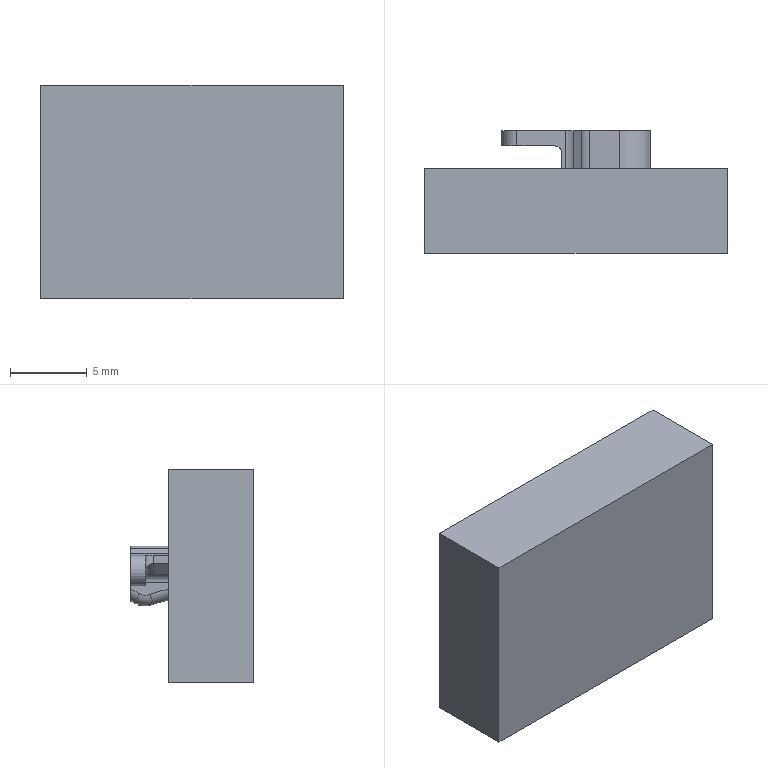NC program | NX | posted with a generic post | part box 19.7 x 8 x 13.91 mm
Lines 6971 to 7835 of 12778:
(ZLEVEL_PROFILE_COPY_1 , TOOL : D2)
N13910 T02 M6
N13912 G54
N13914 G17 G0 G90 X1.619 Y-2.755 B0. C0. S6500 M3
N13916 G43 Z30. H2
N13918 Z-0.04
N13920 G94 G1 X1.446 Y-2.455 F1000.
N13922 G3 X1.273 Y-2.355 R0.2
N13924 G1 X0.696 F1200.
N13926 X0.202 Y-2.652
N13928 G3 X0.105 Y-2.826 R0.2
N13930 G1 X0.111 Y-3.151
N13932 G0 X1.619 Y-2.755 Z-0.08
N13934 G1 X1.446 Y-2.455 F1000.
N13936 G3 X1.273 Y-2.355 R0.2
N13938 G1 X0.696 F1200.
N13940 X0.202 Y-2.652
N13942 G3 X0.105 Y-2.826 R0.2
N13944 G1 X0.111 Y-3.151
N13946 G0 X1.619 Y-2.755 Z-0.12
N13948 G1 X1.446 Y-2.455 F1000.
N13950 G3 X1.273 Y-2.355 R0.2
N13952 G1 X0.696 F1200.
N13954 X0.202 Y-2.652
N13956 G3 X0.105 Y-2.826 R0.2
N13958 G1 X0.111 Y-3.151
N13960 G0 X1.619 Y-2.755 Z-0.16
N13962 G1 X1.446 Y-2.455 F1000.
N13964 G3 X1.273 Y-2.355 R0.2
N13966 G1 X0.696 F1200.
N13968 X0.202 Y-2.652
N13970 G3 X0.105 Y-2.826 R0.2
N13972 G1 X0.111 Y-3.151
N13974 G0 X1.619 Y-2.755 Z-0.2
N13976 G1 X1.446 Y-2.455 F1000.
N13978 G3 X1.273 Y-2.355 R0.2
N13980 G1 X0.696 F1200.
N13982 X0.202 Y-2.652
N13984 G3 X0.105 Y-2.826 R0.2
N13986 G1 X0.111 Y-3.151
N13988 G0 X1.619 Y-2.755 Z-0.24
N13990 G1 X1.446 Y-2.455 F1000.
N13992 G3 X1.273 Y-2.355 R0.2
N13994 G1 X0.696 F1200.
N13996 X0.202 Y-2.652
N13998 G3 X0.105 Y-2.826 R0.2
N14000 G1 X0.111 Y-3.151
N14002 G0 X1.619 Y-2.755 Z-0.28
N14004 G1 X1.446 Y-2.455 F1000.
N14006 G3 X1.273 Y-2.355 R0.2
N14008 G1 X0.696 F1200.
N14010 X0.202 Y-2.652
N14012 G3 X0.105 Y-2.826 R0.2
N14014 G1 X0.111 Y-3.151
N14016 G0 X1.619 Y-2.755 Z-0.32
N14018 G1 X1.446 Y-2.455 F1000.
N14020 G3 X1.273 Y-2.355 R0.2
N14022 G1 X0.696 F1200.
N14024 X0.202 Y-2.652
N14026 G3 X0.105 Y-2.826 R0.2
N14028 G1 X0.111 Y-3.151
N14030 G0 X1.619 Y-2.755 Z-0.36
N14032 G1 X1.446 Y-2.455 F1000.
N14034 G3 X1.273 Y-2.355 R0.2
N14036 G1 X0.696 F1200.
N14038 X0.202 Y-2.652
N14040 G3 X0.105 Y-2.826 R0.2
N14042 G1 X0.111 Y-3.151
N14044 G0 X1.619 Y-2.755 Z-0.4
N14046 G1 X1.446 Y-2.455 F1000.
N14048 G3 X1.273 Y-2.355 R0.2
N14050 G1 X0.696 F1200.
N14052 X0.202 Y-2.652
N14054 G3 X0.105 Y-2.826 R0.2
N14056 G1 X0.111 Y-3.151
N14058 G0 X1.619 Y-2.755 Z-0.44
N14060 G1 X1.446 Y-2.455 F1000.
N14062 G3 X1.273 Y-2.355 R0.2
N14064 G1 X0.696 F1200.
N14066 X0.202 Y-2.652
N14068 G3 X0.105 Y-2.826 R0.2
N14070 G1 X0.111 Y-3.151
N14072 G0 X1.619 Y-2.755 Z-0.48
N14074 G1 X1.446 Y-2.455 F1000.
N14076 G3 X1.273 Y-2.355 R0.2
N14078 G1 X0.696 F1200.
N14080 X0.202 Y-2.652
N14082 G3 X0.105 Y-2.826 R0.2
N14084 G1 X0.111 Y-3.151
N14086 G0 X1.619 Y-2.755 Z-0.52
N14088 G1 X1.446 Y-2.455 F1000.
N14090 G3 X1.273 Y-2.355 R0.2
N14092 G1 X0.696 F1200.
N14094 X0.202 Y-2.652
N14096 G3 X0.105 Y-2.826 R0.2
N14098 G1 X0.111 Y-3.151
N14100 G0 X1.619 Y-2.755 Z-0.56
N14102 G1 X1.446 Y-2.455 F1000.
N14104 G3 X1.273 Y-2.355 R0.2
N14106 G1 X0.696 F1200.
N14108 X0.202 Y-2.652
N14110 G3 X0.105 Y-2.826 R0.2
N14112 G1 X0.111 Y-3.151
N14114 G0 X1.619 Y-2.755 Z-0.6
N14116 G1 X1.446 Y-2.455 F1000.
N14118 G3 X1.273 Y-2.355 R0.2
N14120 G1 X0.696 F1200.
N14122 X0.202 Y-2.652
N14124 G3 X0.105 Y-2.826 R0.2
N14126 G1 X0.111 Y-3.151
N14128 G0 X1.619 Y-2.755 Z-0.64
N14130 G1 X1.446 Y-2.455 F1000.
N14132 G3 X1.273 Y-2.355 R0.2
N14134 G1 X0.696 F1200.
N14136 X0.202 Y-2.652
N14138 G3 X0.105 Y-2.826 R0.2
N14140 G1 X0.111 Y-3.151
N14142 G0 X1.619 Y-2.755 Z-0.68
N14144 G1 X1.446 Y-2.455 F1000.
N14146 G3 X1.273 Y-2.355 R0.2
N14148 G1 X0.696 F1200.
N14150 X0.202 Y-2.652
N14152 G3 X0.105 Y-2.826 R0.2
N14154 G1 X0.111 Y-3.151
N14156 G0 X1.619 Y-2.755 Z-0.72
N14158 G1 X1.446 Y-2.455 F1000.
N14160 G3 X1.273 Y-2.355 R0.2
N14162 G1 X0.696 F1200.
N14164 X0.202 Y-2.652
N14166 G3 X0.105 Y-2.826 R0.2
N14168 G1 X0.111 Y-3.151
N14170 G0 X1.619 Y-2.755 Z-0.76
N14172 G1 X1.446 Y-2.455 F1000.
N14174 G3 X1.273 Y-2.355 R0.2
N14176 G1 X0.696 F1200.
N14178 X0.202 Y-2.652
N14180 G3 X0.105 Y-2.826 R0.2
N14182 G1 X0.111 Y-3.151
N14184 G0 X1.619 Y-2.755 Z-0.8
N14186 G1 X1.446 Y-2.455 F1000.
N14188 G3 X1.273 Y-2.355 R0.2
N14190 G1 X0.696 F1200.
N14192 X0.202 Y-2.652
N14194 G3 X0.105 Y-2.826 R0.2
N14196 G1 X0.111 Y-3.151
N14198 G0 X1.619 Y-2.755 Z-0.84
N14200 G1 X1.446 Y-2.455 F1000.
N14202 G3 X1.273 Y-2.355 R0.2
N14204 G1 X0.696 F1200.
N14206 X0.202 Y-2.652
N14208 G3 X0.105 Y-2.826 R0.2
N14210 G1 X0.111 Y-3.151
N14212 G0 X1.619 Y-2.755 Z-0.88
N14214 G1 X1.446 Y-2.455 F1000.
N14216 G3 X1.273 Y-2.355 R0.2
N14218 G1 X0.696 F1200.
N14220 X0.202 Y-2.652
N14222 G3 X0.105 Y-2.826 R0.2
N14224 G1 X0.111 Y-3.151
N14226 G0 X1.619 Y-2.755 Z-0.92
N14228 G1 X1.446 Y-2.455 F1000.
N14230 G3 X1.273 Y-2.355 R0.2
N14232 G1 X0.696 F1200.
N14234 X0.202 Y-2.652
N14236 G3 X0.105 Y-2.826 R0.2
N14238 G1 X0.111 Y-3.151
N14240 G0 X1.619 Y-2.755 Z-0.96
N14242 G1 X1.446 Y-2.455 F1000.
N14244 G3 X1.273 Y-2.355 R0.2
N14246 G1 X0.696 F1200.
N14248 X0.202 Y-2.652
N14250 G3 X0.105 Y-2.826 R0.2
N14252 G1 X0.111 Y-3.151
N14254 G0 X1.619 Y-2.755 Z-1.
N14256 G1 X1.446 Y-2.455 F1000.
N14258 G3 X1.273 Y-2.355 R0.2
N14260 G1 X0.696 F1200.
N14262 X0.202 Y-2.652
N14264 G3 X0.105 Y-2.826 R0.2
N14266 G1 X0.111 Y-3.151
N14268 G0 X1.619 Y-2.755 Z-1.04
N14270 G1 X1.446 Y-2.455 F1000.
N14272 G3 X1.273 Y-2.355 R0.2
N14274 G1 X0.696 F1200.
N14276 X0.202 Y-2.652
N14278 G3 X0.105 Y-2.826 R0.2
N14280 G1 X0.111 Y-3.151
N14282 G0 X1.619 Y-2.755 Z-1.08
N14284 G1 X1.446 Y-2.455 F1000.
N14286 G3 X1.273 Y-2.355 R0.2
N14288 G1 X0.696 F1200.
N14290 X0.202 Y-2.652
N14292 G3 X0.105 Y-2.826 R0.2
N14294 G1 X0.111 Y-3.151
N14296 G0 X1.619 Y-2.755 Z-1.12
N14298 G1 X1.446 Y-2.455 F1000.
N14300 G3 X1.273 Y-2.355 R0.2
N14302 G1 X0.696 F1200.
N14304 X0.202 Y-2.652
N14306 G3 X0.105 Y-2.826 R0.2
N14308 G1 X0.111 Y-3.151
N14310 G0 X1.619 Y-2.755 Z-1.16
N14312 G1 X1.446 Y-2.455 F1000.
N14314 G3 X1.273 Y-2.355 R0.2
N14316 G1 X0.696 F1200.
N14318 X0.202 Y-2.652
N14320 G3 X0.105 Y-2.826 R0.2
N14322 G1 X0.111 Y-3.151
N14324 G0 X1.619 Y-2.755 Z-1.2
N14326 G1 X1.446 Y-2.455 F1000.
N14328 G3 X1.273 Y-2.355 R0.2
N14330 G1 X0.696 F1200.
N14332 X0.202 Y-2.652
N14334 G3 X0.105 Y-2.826 R0.2
N14336 G1 X0.111 Y-3.151
N14338 G0 X1.619 Y-2.755 Z-1.24
N14340 G1 X1.446 Y-2.455 F1000.
N14342 G3 X1.273 Y-2.355 R0.2
N14344 G1 X0.696 F1200.
N14346 X0.202 Y-2.652
N14348 G3 X0.105 Y-2.826 R0.2
N14350 G1 X0.111 Y-3.151
N14352 G0 X1.619 Y-2.755 Z-1.28
N14354 G1 X1.446 Y-2.455 F1000.
N14356 G3 X1.273 Y-2.355 R0.2
N14358 G1 X0.696 F1200.
N14360 X0.202 Y-2.652
N14362 G3 X0.105 Y-2.826 R0.2
N14364 G1 X0.111 Y-3.151
N14366 G0 X1.619 Y-2.755 Z-1.32
N14368 G1 X1.446 Y-2.455 F1000.
N14370 G3 X1.273 Y-2.355 R0.2
N14372 G1 X0.696 F1200.
N14374 X0.202 Y-2.652
N14376 G3 X0.105 Y-2.826 R0.2
N14378 G1 X0.111 Y-3.151
N14380 G0 X1.619 Y-2.755 Z-1.36
N14382 G1 X1.446 Y-2.455 F1000.
N14384 G3 X1.273 Y-2.355 R0.2
N14386 G1 X0.696 F1200.
N14388 X0.202 Y-2.652
N14390 G3 X0.105 Y-2.826 R0.2
N14392 G1 X0.111 Y-3.151
N14394 G0 X1.619 Y-2.755 Z-1.4
N14396 G1 X1.446 Y-2.455 F1000.
N14398 G3 X1.273 Y-2.355 R0.2
N14400 G1 X0.696 F1200.
N14402 X0.202 Y-2.652
N14404 G3 X0.105 Y-2.826 R0.2
N14406 G1 X0.111 Y-3.151
N14408 G0 X1.619 Y-2.755 Z-1.44
N14410 G1 X1.446 Y-2.455 F1000.
N14412 G3 X1.273 Y-2.355 R0.2
N14414 G1 X0.696 F1200.
N14416 X0.202 Y-2.652
N14418 G3 X0.105 Y-2.826 R0.2
N14420 G1 X0.111 Y-3.151
N14422 G0 X1.619 Y-2.755 Z-1.48
N14424 G1 X1.446 Y-2.455 F1000.
N14426 G3 X1.273 Y-2.355 R0.2
N14428 G1 X0.696 F1200.
N14430 X0.202 Y-2.652
N14432 G3 X0.105 Y-2.826 R0.2
N14434 G1 X0.111 Y-3.151
N14436 G0 X1.619 Y-2.755 Z-1.52
N14438 G1 X1.446 Y-2.455 F1000.
N14440 G3 X1.273 Y-2.355 R0.2
N14442 G1 X0.696 F1200.
N14444 X0.202 Y-2.652
N14446 G3 X0.105 Y-2.826 R0.2
N14448 G1 X0.111 Y-3.151
N14450 G0 X1.619 Y-2.755 Z-1.56
N14452 G1 X1.446 Y-2.455 F1000.
N14454 G3 X1.273 Y-2.355 R0.2
N14456 G1 X0.696 F1200.
N14458 X0.202 Y-2.652
N14460 G3 X0.105 Y-2.826 R0.2
N14462 G1 X0.111 Y-3.151
N14464 G0 X1.619 Y-2.755 Z-1.6
N14466 G1 X1.446 Y-2.455 F1000.
N14468 G3 X1.273 Y-2.355 R0.2
N14470 G1 X0.696 F1200.
N14472 X0.202 Y-2.652
N14474 G3 X0.105 Y-2.826 R0.2
N14476 G1 X0.111 Y-3.151
N14478 G0 X1.619 Y-2.755 Z-1.64
N14480 G1 X1.446 Y-2.455 F1000.
N14482 G3 X1.273 Y-2.355 R0.2
N14484 G1 X0.696 F1200.
N14486 X0.202 Y-2.652
N14488 G3 X0.105 Y-2.826 R0.2
N14490 G1 X0.111 Y-3.151
N14492 G0 X1.619 Y-2.755 Z-1.68
N14494 G1 X1.446 Y-2.455 F1000.
N14496 G3 X1.273 Y-2.355 R0.2
N14498 G1 X0.696 F1200.
N14500 X0.202 Y-2.652
N14502 G3 X0.105 Y-2.826 R0.2
N14504 G1 X0.111 Y-3.151
N14506 G0 X1.619 Y-2.755 Z-1.72
N14508 G1 X1.446 Y-2.455 F1000.
N14510 G3 X1.273 Y-2.355 R0.2
N14512 G1 X0.696 F1200.
N14514 X0.202 Y-2.652
N14516 G3 X0.105 Y-2.826 R0.2
N14518 G1 X0.111 Y-3.151
N14520 G0 X1.619 Y-2.755 Z-1.76
N14522 G1 X1.446 Y-2.455 F1000.
N14524 G3 X1.273 Y-2.355 R0.2
N14526 G1 X0.696 F1200.
N14528 X0.202 Y-2.652
N14530 G3 X0.105 Y-2.826 R0.2
N14532 G1 X0.111 Y-3.151
N14534 G0 X1.619 Y-2.755 Z-1.8
N14536 G1 X1.446 Y-2.455 F1000.
N14538 G3 X1.273 Y-2.355 R0.2
N14540 G1 X0.696 F1200.
N14542 X0.202 Y-2.652
N14544 G3 X0.105 Y-2.826 R0.2
N14546 G1 X0.111 Y-3.151
N14548 G0 X1.619 Y-2.755 Z-1.84
N14550 G1 X1.446 Y-2.455 F1000.
N14552 G3 X1.273 Y-2.355 R0.2
N14554 G1 X0.696 F1200.
N14556 X0.202 Y-2.652
N14558 G3 X0.105 Y-2.826 R0.2
N14560 G1 X0.111 Y-3.151
N14562 G0 X1.619 Y-2.755 Z-1.88
N14564 G1 X1.446 Y-2.455 F1000.
N14566 G3 X1.273 Y-2.355 R0.2
N14568 G1 X0.696 F1200.
N14570 X0.202 Y-2.652
N14572 G3 X0.105 Y-2.826 R0.2
N14574 G1 X0.111 Y-3.151
N14576 G0 X1.619 Y-2.755 Z-1.92
N14578 G1 X1.446 Y-2.455 F1000.
N14580 G3 X1.273 Y-2.355 R0.2
N14582 G1 X0.696 F1200.
N14584 X0.202 Y-2.652
N14586 G3 X0.105 Y-2.826 R0.2
N14588 G1 X0.111 Y-3.151
N14590 G0 X1.619 Y-2.755 Z-1.96
N14592 G1 X1.446 Y-2.455 F1000.
N14594 G3 X1.273 Y-2.355 R0.2
N14596 G1 X0.696 F1200.
N14598 X0.202 Y-2.652
N14600 G3 X0.105 Y-2.826 R0.2
N14602 G1 X0.111 Y-3.151
N14604 G0 X1.619 Y-2.755 Z-2.
N14606 G1 X1.446 Y-2.455 F1000.
N14608 G3 X1.273 Y-2.355 R0.2
N14610 G1 X0.696 F1200.
N14612 X0.202 Y-2.652
N14614 G3 X0.105 Y-2.826 R0.2
N14616 G1 X0.111 Y-3.151
N14618 G0 X1.619 Y-2.755 Z-2.04
N14620 G1 X1.446 Y-2.455 F1000.
N14622 G3 X1.273 Y-2.355 R0.2
N14624 G1 X0.696 F1200.
N14626 X0.202 Y-2.652
N14628 G3 X0.105 Y-2.826 R0.2
N14630 G1 X0.111 Y-3.151
N14632 G0 X1.619 Y-2.755 Z-2.08
N14634 G1 X1.446 Y-2.455 F1000.
N14636 G3 X1.273 Y-2.355 R0.2
N14638 G1 X0.696 F1200.
N14640 X0.202 Y-2.652
N14642 G3 X0.105 Y-2.826 R0.2
N14644 G1 X0.111 Y-3.151
N14646 G0 X1.619 Y-2.755 Z-2.12
N14648 G1 X1.446 Y-2.455 F1000.
N14650 G3 X1.273 Y-2.355 R0.2
N14652 G1 X0.696 F1200.
N14654 X0.202 Y-2.652
N14656 G3 X0.105 Y-2.826 R0.2
N14658 G1 X0.111 Y-3.151
N14660 G0 X1.619 Y-2.755 Z-2.16
N14662 G1 X1.446 Y-2.455 F1000.
N14664 G3 X1.273 Y-2.355 R0.2
N14666 G1 X0.696 F1200.
N14668 X0.202 Y-2.652
N14670 G3 X0.105 Y-2.826 R0.2
N14672 G1 X0.111 Y-3.151
N14674 G0 X1.619 Y-2.755 Z-2.2
N14676 G1 X1.446 Y-2.455 F1000.
N14678 G3 X1.273 Y-2.355 R0.2
N14680 G1 X0.696 F1200.
N14682 X0.202 Y-2.652
N14684 G3 X0.105 Y-2.826 R0.2
N14686 G1 X0.111 Y-3.151
N14688 G0 X1.619 Y-2.755 Z-2.24
N14690 G1 X1.446 Y-2.455 F1000.
N14692 G3 X1.273 Y-2.355 R0.2
N14694 G1 X0.696 F1200.
N14696 X0.202 Y-2.652
N14698 G3 X0.105 Y-2.826 R0.2
N14700 G1 X0.111 Y-3.151
N14702 G0 X1.619 Y-2.755 Z-2.28
N14704 G1 X1.446 Y-2.455 F1000.
N14706 G3 X1.273 Y-2.355 R0.2
N14708 G1 X0.696 F1200.
N14710 X0.202 Y-2.652
N14712 G3 X0.105 Y-2.826 R0.2
N14714 G1 X0.111 Y-3.151
N14716 G0 X1.619 Y-2.755 Z-2.32
N14718 G1 X1.446 Y-2.455 F1000.
N14720 G3 X1.273 Y-2.355 R0.2
N14722 G1 X0.696 F1200.
N14724 X0.202 Y-2.652
N14726 G3 X0.105 Y-2.826 R0.2
N14728 G1 X0.111 Y-3.151
N14730 G0 X1.619 Y-2.755 Z-2.36
N14732 G1 X1.446 Y-2.455 F1000.
N14734 G3 X1.273 Y-2.355 R0.2
N14736 G1 X0.696 F1200.
N14738 X0.202 Y-2.652
N14740 G3 X0.105 Y-2.826 R0.2
N14742 G1 X0.111 Y-3.151
N14744 G0 X1.619 Y-2.755 Z-2.4
N14746 G1 X1.446 Y-2.455 F1000.
N14748 G3 X1.273 Y-2.355 R0.2
N14750 G1 X0.696 F1200.
N14752 X0.202 Y-2.652
N14754 G3 X0.105 Y-2.826 R0.2
N14756 G1 X0.111 Y-3.151
N14758 G0 X1.619 Y-2.755 Z-2.44
N14760 G1 X1.446 Y-2.455 F1000.
N14762 G3 X1.273 Y-2.355 R0.2
N14764 G1 X0.696 F1200.
N14766 X0.202 Y-2.652
N14768 G3 X0.105 Y-2.826 R0.2
N14770 G1 X0.111 Y-3.151
N14772 G0 X1.619 Y-2.755 Z-2.48
N14774 G1 X1.446 Y-2.455 F1000.
N14776 G3 X1.273 Y-2.355 R0.2
N14778 G1 X0.696 F1200.
N14780 X0.202 Y-2.652
N14782 G3 X0.105 Y-2.826 R0.2
N14784 G1 X0.111 Y-3.151
N14786 G0 X1.619 Y-2.755 Z-2.52
N14788 G1 X1.446 Y-2.455 F1000.
N14790 G3 X1.273 Y-2.355 R0.2
N14792 G1 X0.696 F1200.
N14794 X0.202 Y-2.652
N14796 G3 X0.105 Y-2.826 R0.2
N14798 G1 X0.111 Y-3.151
N14800 G0 X1.619 Y-2.755 Z-2.56
N14802 G1 X1.446 Y-2.455 F1000.
N14804 G3 X1.273 Y-2.355 R0.2
N14806 G1 X0.696 F1200.
N14808 X0.202 Y-2.652
N14810 G3 X0.105 Y-2.826 R0.2
N14812 G1 X0.111 Y-3.151
N14814 G0 X1.619 Y-2.755 Z-2.6
N14816 G1 X1.446 Y-2.455 F1000.
N14818 G3 X1.273 Y-2.355 R0.2
N14820 G1 X0.696 F1200.
N14822 X0.202 Y-2.652
N14824 G3 X0.105 Y-2.826 R0.2
N14826 G1 X0.111 Y-3.151
N14828 G0 X1.619 Y-2.755 Z-2.64
N14830 G1 X1.446 Y-2.455 F1000.
N14832 G3 X1.273 Y-2.355 R0.2
N14834 G1 X0.696 F1200.
N14836 X0.202 Y-2.652
N14838 G3 X0.105 Y-2.826 R0.2
N14840 G1 X0.111 Y-3.151
N14842 G0 X1.619 Y-2.755 Z-2.68
N14844 G1 X1.446 Y-2.455 F1000.
N14846 G3 X1.273 Y-2.355 R0.2
N14848 G1 X0.696 F1200.
N14850 X0.202 Y-2.652
N14852 G3 X0.105 Y-2.826 R0.2
N14854 G1 X0.111 Y-3.151
N14856 G0 X1.619 Y-2.755 Z-2.72
N14858 G1 X1.446 Y-2.455 F1000.
N14860 G3 X1.273 Y-2.355 R0.2
N14862 G1 X0.696 F1200.
N14864 X0.202 Y-2.652
N14866 G3 X0.105 Y-2.826 R0.2
N14868 G1 X0.111 Y-3.151
N14870 G0 X1.619 Y-2.755 Z-2.76
N14872 G1 X1.446 Y-2.455 F1000.
N14874 G3 X1.273 Y-2.355 R0.2
N14876 G1 X0.696 F1200.
N14878 X0.202 Y-2.652
N14880 G3 X0.105 Y-2.826 R0.2
N14882 G1 X0.111 Y-3.151
N14884 G0 X1.619 Y-2.755 Z-2.8
N14886 G1 X1.446 Y-2.455 F1000.
N14888 G3 X1.273 Y-2.355 R0.2
N14890 G1 X0.696 F1200.
N14892 X0.202 Y-2.652
N14894 G3 X0.105 Y-2.826 R0.2
N14896 G1 X0.111 Y-3.151
N14898 G0 X1.619 Y-2.755 Z-2.84
N14900 G1 X1.446 Y-2.455 F1000.
N14902 G3 X1.273 Y-2.355 R0.2
N14904 G1 X0.696 F1200.
N14906 X0.202 Y-2.652
N14908 G3 X0.105 Y-2.826 R0.2
N14910 G1 X0.111 Y-3.151
N14912 G0 X1.619 Y-2.755 Z-2.88
N14914 G1 X1.446 Y-2.455 F1000.
N14916 G3 X1.273 Y-2.355 R0.2
N14918 G1 X0.696 F1200.
N14920 X0.202 Y-2.652
N14922 G3 X0.105 Y-2.826 R0.2
N14924 G1 X0.111 Y-3.151
N14926 G0 X1.619 Y-2.755 Z-2.92
N14928 G1 X1.446 Y-2.455 F1000.
N14930 G3 X1.273 Y-2.355 R0.2
N14932 G1 X0.696 F1200.
N14934 X0.202 Y-2.652
N14936 G3 X0.105 Y-2.826 R0.2
N14938 G1 X0.111 Y-3.151
N14940 G0 X1.619 Y-2.755 Z-2.96
N14942 G1 X1.446 Y-2.455 F1000.
N14944 G3 X1.273 Y-2.355 R0.2
N14946 G1 X0.696 F1200.
N14948 X0.202 Y-2.652
N14950 G3 X0.105 Y-2.826 R0.2
N14952 G1 X0.111 Y-3.151
N14954 G0 X1.619 Y-2.755 Z-3.
N14956 G1 X1.446 Y-2.455 F1000.
N14958 G3 X1.273 Y-2.355 R0.2
N14960 G1 X0.696 F1200.
N14962 X0.202 Y-2.652
N14964 G3 X0.105 Y-2.826 R0.2
N14966 G1 X0.111 Y-3.151
N14968 G0 X1.619 Y-2.755 Z-3.04
N14970 G1 X1.446 Y-2.455 F1000.
N14972 G3 X1.273 Y-2.355 R0.2
N14974 G1 X0.696 F1200.
N14976 X0.202 Y-2.652
N14978 G3 X0.105 Y-2.826 R0.2
N14980 G1 X0.111 Y-3.151
N14982 G0 X1.619 Y-2.755 Z-3.08
N14984 G1 X1.446 Y-2.455 F1000.
N14986 G3 X1.273 Y-2.355 R0.2
N14988 G1 X0.696 F1200.
N14990 X0.202 Y-2.652
N14992 G3 X0.105 Y-2.826 R0.2
N14994 G1 X0.111 Y-3.151
N14996 G0 X1.619 Y-2.755 Z-3.12
N14998 G1 X1.446 Y-2.455 F1000.
N15000 G3 X1.273 Y-2.355 R0.2
N15002 G1 X0.696 F1200.
N15004 X0.202 Y-2.652
N15006 G3 X0.105 Y-2.826 R0.2
N15008 G1 X0.111 Y-3.151
N15010 G0 X1.619 Y-2.755 Z-3.16
N15012 G1 X1.446 Y-2.455 F1000.
N15014 G3 X1.273 Y-2.355 R0.2
N15016 G1 X0.696 F1200.
N15018 X0.202 Y-2.652
N15020 G3 X0.105 Y-2.826 R0.2
N15022 G1 X0.111 Y-3.151
N15024 G0 X1.619 Y-2.755 Z-3.2
N15026 G1 X1.446 Y-2.455 F1000.
N15028 G3 X1.273 Y-2.355 R0.2
N15030 G1 X0.696 F1200.
N15032 X0.202 Y-2.652
N15034 G3 X0.105 Y-2.826 R0.2
N15036 G1 X0.111 Y-3.151
N15038 G0 X1.619 Y-2.755 Z-3.24
N15040 G1 X1.446 Y-2.455 F1000.
N15042 G3 X1.273 Y-2.355 R0.2
N15044 G1 X0.696 F1200.
N15046 X0.202 Y-2.652
N15048 G3 X0.105 Y-2.826 R0.2
N15050 G1 X0.111 Y-3.151
N15052 G0 X1.619 Y-2.755 Z-3.28
N15054 G1 X1.446 Y-2.455 F1000.
N15056 G3 X1.273 Y-2.355 R0.2
N15058 G1 X0.696 F1200.
N15060 X0.202 Y-2.652
N15062 G3 X0.105 Y-2.826 R0.2
N15064 G1 X0.111 Y-3.151
N15066 G0 X1.619 Y-2.755 Z-3.32
N15068 G1 X1.446 Y-2.455 F1000.
N15070 G3 X1.273 Y-2.355 R0.2
N15072 G1 X0.696 F1200.
N15074 X0.202 Y-2.652
N15076 G3 X0.105 Y-2.826 R0.2
N15078 G1 X0.111 Y-3.151
N15080 G0 X1.619 Y-2.755 Z-3.36
N15082 G1 X1.446 Y-2.455 F1000.
N15084 G3 X1.273 Y-2.355 R0.2
N15086 G1 X0.696 F1200.
N15088 X0.202 Y-2.652
N15090 G3 X0.105 Y-2.826 R0.2
N15092 G1 X0.111 Y-3.151
N15094 G0 X1.619 Y-2.755 Z-3.4
N15096 G1 X1.446 Y-2.455 F1000.
N15098 G3 X1.273 Y-2.355 R0.2
N15100 G1 X0.696 F1200.
N15102 X0.202 Y-2.652
N15104 G3 X0.105 Y-2.826 R0.2
N15106 G1 X0.111 Y-3.151
N15108 G0 X1.619 Y-2.755 Z-3.44
N15110 G1 X1.446 Y-2.455 F1000.
N15112 G3 X1.273 Y-2.355 R0.2
N15114 G1 X0.696 F1200.
N15116 X0.202 Y-2.652
N15118 G3 X0.105 Y-2.826 R0.2
N15120 G1 X0.111 Y-3.151
N15122 G0 X1.619 Y-2.755 Z-3.48
N15124 G1 X1.446 Y-2.455 F1000.
N15126 G3 X1.273 Y-2.355 R0.2
N15128 G1 X0.696 F1200.
N15130 X0.202 Y-2.652
N15132 G3 X0.105 Y-2.826 R0.2
N15134 G1 X0.111 Y-3.151
N15136 G0 X1.619 Y-2.755 Z-3.52
N15138 G1 X1.446 Y-2.455 F1000.
N15140 G3 X1.273 Y-2.355 R0.2
N15142 G1 X0.696 F1200.
N15144 X0.202 Y-2.652
N15146 G3 X0.105 Y-2.826 R0.2
N15148 G1 X0.111 Y-3.151
N15150 G0 X1.619 Y-2.755 Z-3.56
N15152 G1 X1.446 Y-2.455 F1000.
N15154 G3 X1.273 Y-2.355 R0.2
N15156 G1 X0.696 F1200.
N15158 X0.202 Y-2.652
N15160 G3 X0.105 Y-2.826 R0.2
N15162 G1 X0.111 Y-3.151
N15164 G0 X1.619 Y-2.755 Z-3.6
N15166 G1 X1.446 Y-2.455 F1000.
N15168 G3 X1.273 Y-2.355 R0.2
N15170 G1 X0.696 F1200.
N15172 X0.202 Y-2.652
N15174 G3 X0.105 Y-2.826 R0.2
N15176 G1 X0.111 Y-3.151
N15178 G0 X1.619 Y-2.755 Z-3.64
N15180 G1 X1.446 Y-2.455 F1000.
N15182 G3 X1.273 Y-2.355 R0.2
N15184 G1 X0.696 F1200.
N15186 X0.202 Y-2.652
N15188 G3 X0.105 Y-2.826 R0.2
N15190 G1 X0.111 Y-3.151
N15192 G0 X1.619 Y-2.755 Z-3.68
N15194 G1 X1.446 Y-2.455 F1000.
N15196 G3 X1.273 Y-2.355 R0.2
N15198 G1 X0.696 F1200.
N15200 X0.202 Y-2.652
N15202 G3 X0.105 Y-2.826 R0.2
N15204 G1 X0.111 Y-3.151
N15206 G0 X1.619 Y-2.755 Z-3.72
N15208 G1 X1.446 Y-2.455 F1000.
N15210 G3 X1.273 Y-2.355 R0.2
N15212 G1 X0.696 F1200.
N15214 X0.202 Y-2.652
N15216 G3 X0.105 Y-2.826 R0.2
N15218 G1 X0.111 Y-3.151
N15220 G0 X1.619 Y-2.755 Z-3.76
N15222 G1 X1.446 Y-2.455 F1000.
N15224 G3 X1.273 Y-2.355 R0.2
N15226 G1 X0.696 F1200.
N15228 X0.202 Y-2.652
N15230 G3 X0.105 Y-2.826 R0.2
N15232 G1 X0.111 Y-3.151
N15234 G0 X1.619 Y-2.755 Z-3.8
N15236 G1 X1.446 Y-2.455 F1000.
N15238 G3 X1.273 Y-2.355 R0.2
N15240 G1 X0.696 F1200.
N15242 X0.202 Y-2.652
N15244 G3 X0.105 Y-2.826 R0.2
N15246 G1 X0.111 Y-3.151
N15248 G0 X1.619 Y-2.755 Z-3.84
N15250 G1 X1.446 Y-2.455 F1000.
N15252 G3 X1.273 Y-2.355 R0.2
N15254 G1 X0.696 F1200.
N15256 X0.202 Y-2.652
N15258 G3 X0.105 Y-2.826 R0.2
N15260 G1 X0.111 Y-3.151
N15262 G0 X1.619 Y-2.755 Z-3.88
N15264 G1 X1.446 Y-2.455 F1000.
N15266 G3 X1.273 Y-2.355 R0.2
N15268 G1 X0.696 F1200.
N15270 X0.202 Y-2.652
N15272 G3 X0.105 Y-2.826 R0.2
N15274 G1 X0.111 Y-3.151
N15276 G0 X1.619 Y-2.755 Z-3.92
N15278 G1 X1.446 Y-2.455 F1000.
N15280 G3 X1.273 Y-2.355 R0.2
N15282 G1 X0.696 F1200.
N15284 X0.202 Y-2.652
N15286 G3 X0.105 Y-2.826 R0.2
N15288 G1 X0.111 Y-3.151
N15290 G0 X1.619 Y-2.755 Z-3.96
N15292 G1 X1.446 Y-2.455 F1000.
N15294 G3 X1.273 Y-2.355 R0.2
N15296 G1 X0.696 F1200.
N15298 X0.202 Y-2.652
N15300 G3 X0.105 Y-2.826 R0.2
N15302 G1 X0.111 Y-3.151
N15304 G0 X1.619 Y-2.755 Z-4.
N15306 G1 X1.446 Y-2.455 F1000.
N15308 G3 X1.273 Y-2.355 R0.2
N15310 G1 X0.696 F1200.
N15312 X0.202 Y-2.652
N15314 G3 X0.105 Y-2.826 R0.2
N15316 G1 X0.111 Y-3.151
N15318 G0 X1.619 Y-2.755 Z-4.04
N15320 G1 X1.446 Y-2.455 F1000.
N15322 G3 X1.273 Y-2.355 R0.2
N15324 G1 X0.696 F1200.
N15326 X0.202 Y-2.652
N15328 G3 X0.105 Y-2.826 R0.2
N15330 G1 X0.111 Y-3.151
N15332 G0 X1.619 Y-2.755 Z-4.08
N15334 G1 X1.446 Y-2.455 F1000.
N15336 G3 X1.273 Y-2.355 R0.2
N15338 G1 X0.696 F1200.
N15340 X0.202 Y-2.652
N15342 G3 X0.105 Y-2.826 R0.2
N15344 G1 X0.111 Y-3.151
N15346 G0 X1.619 Y-2.755 Z-4.12
N15348 G1 X1.446 Y-2.455 F1000.
N15350 G3 X1.273 Y-2.355 R0.2
N15352 G1 X0.696 F1200.
N15354 X0.202 Y-2.652
N15356 G3 X0.105 Y-2.826 R0.2
N15358 G1 X0.111 Y-3.151
N15360 G0 X1.619 Y-2.755 Z-4.16
N15362 G1 X1.446 Y-2.455 F1000.
N15364 G3 X1.273 Y-2.355 R0.2
N15366 G1 X0.696 F1200.
N15368 X0.202 Y-2.652
N15370 G3 X0.105 Y-2.826 R0.2
N15372 G1 X0.111 Y-3.151
N15374 G0 X1.619 Y-2.755 Z-4.2
N15376 G1 X1.446 Y-2.455 F1000.
N15378 G3 X1.273 Y-2.355 R0.2
N15380 G1 X0.696 F1200.
N15382 X0.202 Y-2.652
N15384 G3 X0.105 Y-2.826 R0.2
N15386 G1 X0.111 Y-3.151
N15388 G0 X1.619 Y-2.755 Z-4.24
N15390 G1 X1.446 Y-2.455 F1000.
N15392 G3 X1.273 Y-2.355 R0.2
N15394 G1 X0.696 F1200.
N15396 X0.202 Y-2.652
N15398 G3 X0.105 Y-2.826 R0.2
N15400 G1 X0.111 Y-3.151
N15402 G0 X1.619 Y-2.755 Z-4.28
N15404 G1 X1.446 Y-2.455 F1000.
N15406 G3 X1.273 Y-2.355 R0.2
N15408 G1 X0.696 F1200.
N15410 X0.202 Y-2.652
N15412 G3 X0.105 Y-2.826 R0.2
N15414 G1 X0.111 Y-3.151
N15416 G0 X1.619 Y-2.755 Z-4.32
N15418 G1 X1.446 Y-2.455 F1000.
N15420 G3 X1.273 Y-2.355 R0.2
N15422 G1 X0.696 F1200.
N15424 X0.202 Y-2.652
N15426 G3 X0.105 Y-2.826 R0.2
N15428 G1 X0.111 Y-3.151
N15430 G0 X1.619 Y-2.755 Z-4.36
N15432 G1 X1.446 Y-2.455 F1000.
N15434 G3 X1.273 Y-2.355 R0.2
N15436 G1 X0.696 F1200.
N15438 X0.202 Y-2.652
N15440 G3 X0.105 Y-2.826 R0.2
N15442 G1 X0.111 Y-3.151
N15444 G0 X1.619 Y-2.755 Z-4.4
N15446 G1 X1.446 Y-2.455 F1000.
N15448 G3 X1.273 Y-2.355 R0.2
N15450 G1 X0.696 F1200.
N15452 X0.202 Y-2.652
N15454 G3 X0.105 Y-2.826 R0.2
N15456 G1 X0.111 Y-3.151
N15458 G0 X1.619 Y-2.755 Z-4.44
N15460 G1 X1.446 Y-2.455 F1000.
N15462 G3 X1.273 Y-2.355 R0.2
N15464 G1 X0.696 F1200.
N15466 X0.202 Y-2.652
N15468 G3 X0.105 Y-2.826 R0.2
N15470 G1 X0.111 Y-3.151
N15472 G0 X1.619 Y-2.755 Z-4.48
N15474 G1 X1.446 Y-2.455 F1000.
N15476 G3 X1.273 Y-2.355 R0.2
N15478 G1 X0.696 F1200.
N15480 X0.202 Y-2.652
N15482 G3 X0.105 Y-2.826 R0.2
N15484 G1 X0.111 Y-3.151
N15486 G0 X1.619 Y-2.755 Z-4.52
N15488 G1 X1.446 Y-2.455 F1000.
N15490 G3 X1.273 Y-2.355 R0.2
N15492 G1 X0.696 F1200.
N15494 X0.202 Y-2.652
N15496 G3 X0.105 Y-2.826 R0.2
N15498 G1 X0.111 Y-3.151
N15500 G0 X1.619 Y-2.755 Z-4.56
N15502 G1 X1.446 Y-2.455 F1000.
N15504 G3 X1.273 Y-2.355 R0.2
N15506 G1 X0.696 F1200.
N15508 X0.202 Y-2.652
N15510 G3 X0.105 Y-2.826 R0.2
N15512 G1 X0.111 Y-3.151
N15514 G0 X1.619 Y-2.755 Z-4.6
N15516 G1 X1.446 Y-2.455 F1000.
N15518 G3 X1.273 Y-2.355 R0.2
N15520 G1 X0.696 F1200.
N15522 X0.202 Y-2.652
N15524 G3 X0.105 Y-2.826 R0.2
N15526 G1 X0.111 Y-3.151
N15528 G0 X1.619 Y-2.755 Z-4.64
N15530 G1 X1.446 Y-2.455 F1000.
N15532 G3 X1.273 Y-2.355 R0.2
N15534 G1 X0.696 F1200.
N15536 X0.202 Y-2.652
N15538 G3 X0.105 Y-2.826 R0.2
N15540 G1 X0.111 Y-3.151
N15542 G0 X1.619 Y-2.755 Z-4.68
N15544 G1 X1.446 Y-2.455 F1000.
N15546 G3 X1.273 Y-2.355 R0.2
N15548 G1 X0.696 F1200.
N15550 X0.202 Y-2.652
N15552 G3 X0.105 Y-2.826 R0.2
N15554 G1 X0.111 Y-3.151
N15556 G0 X1.619 Y-2.755 Z-4.72
N15558 G1 X1.446 Y-2.455 F1000.
N15560 G3 X1.273 Y-2.355 R0.2
N15562 G1 X0.696 F1200.
N15564 X0.202 Y-2.652
N15566 G3 X0.105 Y-2.826 R0.2
N15568 G1 X0.111 Y-3.151
N15570 G0 X1.619 Y-2.755 Z-4.76
N15572 G1 X1.446 Y-2.455 F1000.
N15574 G3 X1.273 Y-2.355 R0.2
N15576 G1 X0.696 F1200.
N15578 X0.202 Y-2.652
N15580 G3 X0.105 Y-2.826 R0.2
N15582 G1 X0.111 Y-3.151
N15584 G0 X1.619 Y-2.755 Z-4.8
N15586 G1 X1.446 Y-2.455 F1000.
N15588 G3 X1.273 Y-2.355 R0.2
N15590 G1 X0.696 F1200.
N15592 X0.202 Y-2.652
N15594 G3 X0.105 Y-2.826 R0.2
N15596 G1 X0.111 Y-3.151
N15598 G0 X1.619 Y-2.755 Z-4.84
N15600 G1 X1.446 Y-2.455 F1000.
N15602 G3 X1.273 Y-2.355 R0.2
N15604 G1 X0.696 F1200.
N15606 X0.202 Y-2.652
N15608 G3 X0.105 Y-2.826 R0.2
N15610 G1 X0.111 Y-3.151
N15612 G0 X1.619 Y-2.755 Z-4.88
N15614 G1 X1.446 Y-2.455 F1000.
N15616 G3 X1.273 Y-2.355 R0.2
N15618 G1 X0.696 F1200.
N15620 X0.202 Y-2.652
N15622 G3 X0.105 Y-2.826 R0.2
N15624 G1 X0.111 Y-3.151
N15626 G0 X1.619 Y-2.755 Z-4.92
N15628 G1 X1.446 Y-2.455 F1000.
N15630 G3 X1.273 Y-2.355 R0.2
N15632 G1 X0.696 F1200.